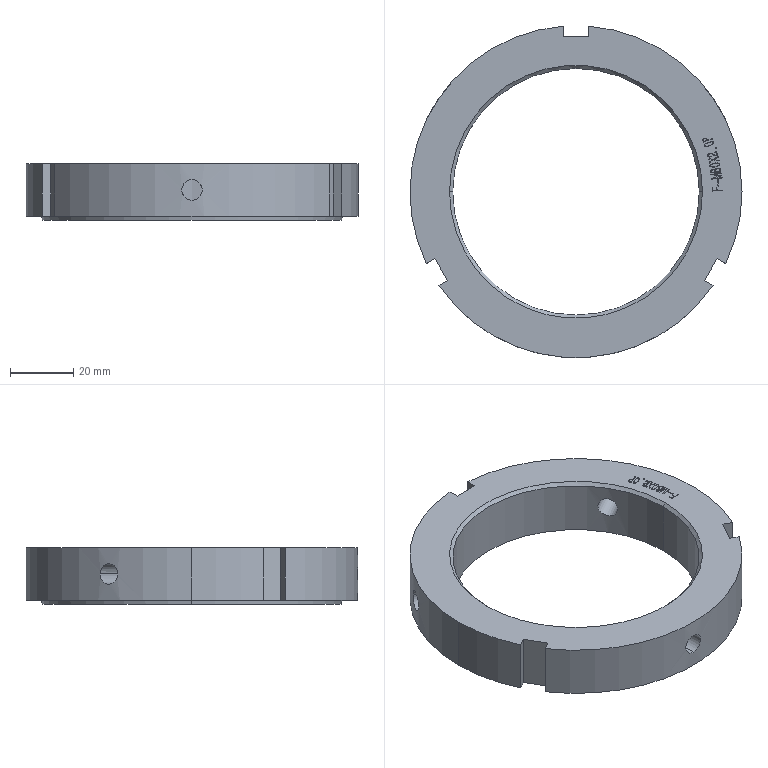Part | STEP file | 7016 Nut 2 | 1 solid | 209 faces | box 105 x 104.847 x 18 mm | volume 64985 mm3 | plane 108 | spline 85 | cylinder 12 | cone 4 | commonest cylinder face diameters 6.5 x6 105 x4 78 x2